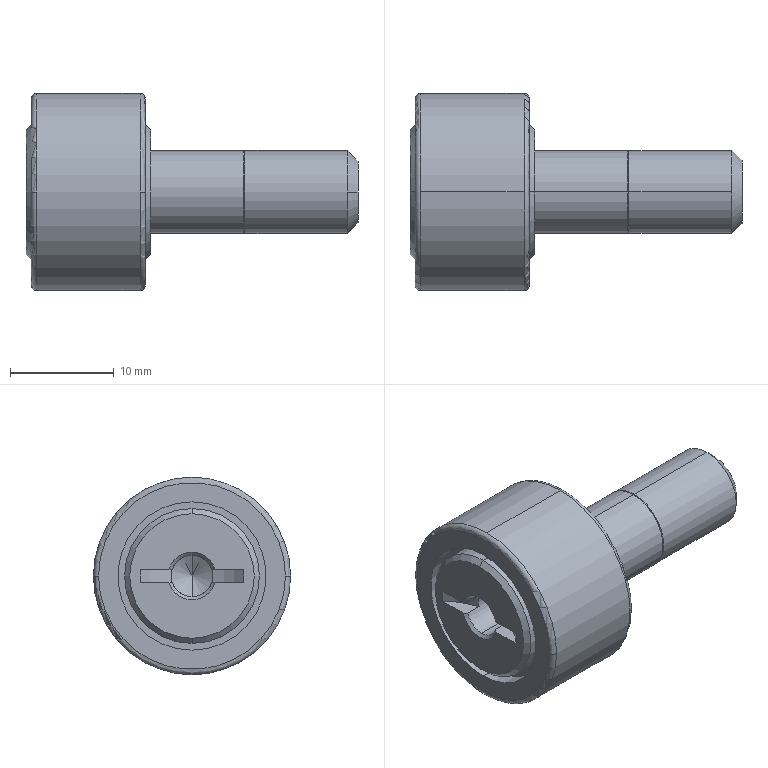Part | NX | 1 solid | 47 faces | box 32 x 19 x 19 mm | volume 4032 mm3 | cylinder 18 | cone 13 | plane 12 | torus 4 | commonest cylinder face diameters 8 x4 13 x4 14.3 x4 4 x2 14 x2 19 x2
STEP:
#1=CARTESIAN_POINT('',(32.,3.,0.));
#2=VERTEX_POINT('',#1);
#3=CARTESIAN_POINT('',(32.,-3.,0.));
#4=VERTEX_POINT('',#3);
#5=CARTESIAN_POINT('',(32.,0.,0.));
#6=DIRECTION('',(1.,0.,0.));
#7=DIRECTION('',(0.,0.,-1.));
#8=AXIS2_PLACEMENT_3D('',#5,#6,#7);
#9=CIRCLE('',#8,3.);
#10=EDGE_CURVE('',#2,#4,#9,.T.);
#11=ORIENTED_EDGE('',*,*,#10,.T.);
#12=CARTESIAN_POINT('',(32.,0.,0.));
#13=DIRECTION('',(1.,0.,0.));
#14=DIRECTION('',(0.,0.,-1.));
#15=AXIS2_PLACEMENT_3D('',#12,#13,#14);
#16=CIRCLE('',#15,3.);
#17=EDGE_CURVE('',#4,#2,#16,.T.);
#18=ORIENTED_EDGE('',*,*,#17,.T.);
#19=EDGE_LOOP('',(#11,#18));
#20=FACE_BOUND('',#19,.T.);
#21=CARTESIAN_POINT('',(32.,0.,0.));
#22=DIRECTION('',(1.,0.,0.));
#23=DIRECTION('',(0.,1.,0.));
#24=AXIS2_PLACEMENT_3D('',#21,#22,#23);
#25=PLANE('',#24);
#26=ADVANCED_FACE('',(#20),#25,.T.);
#27=CARTESIAN_POINT('',(31.,-4.,0.));
#28=VERTEX_POINT('',#27);
#29=CARTESIAN_POINT('',(31.,0.,4.));
#30=VERTEX_POINT('',#29);
#31=CARTESIAN_POINT('',(31.,0.,0.));
#32=DIRECTION('',(-1.,0.,0.));
#33=DIRECTION('',(0.,0.,-1.));
#34=AXIS2_PLACEMENT_3D('',#31,#32,#33);
#35=CIRCLE('',#34,4.);
#36=EDGE_CURVE('',#28,#30,#35,.T.);
#37=ORIENTED_EDGE('',*,*,#36,.F.);
#38=CARTESIAN_POINT('',(31.5,-3.5,0.));
#39=DIRECTION('',(-0.7071,-0.7071,0.));
#40=VECTOR('',#39,1000.);
#41=LINE('',#38,#40);
#42=EDGE_CURVE('',#4,#28,#41,.T.);
#43=ORIENTED_EDGE('',*,*,#42,.F.);
#44=ORIENTED_EDGE('',*,*,#10,.F.);
#45=CARTESIAN_POINT('',(31.,4.,0.));
#46=VERTEX_POINT('',#45);
#47=CARTESIAN_POINT('',(31.5,3.5,0.));
#48=DIRECTION('',(-0.7071,0.7071,0.));
#49=VECTOR('',#48,1000.);
#50=LINE('',#47,#49);
#51=EDGE_CURVE('',#2,#46,#50,.T.);
#52=ORIENTED_EDGE('',*,*,#51,.T.);
#53=CARTESIAN_POINT('',(31.,0.,0.));
#54=DIRECTION('',(-1.,0.,0.));
#55=DIRECTION('',(0.,0.,-1.));
#56=AXIS2_PLACEMENT_3D('',#53,#54,#55);
#57=CIRCLE('',#56,4.);
#58=EDGE_CURVE('',#30,#46,#57,.T.);
#59=ORIENTED_EDGE('',*,*,#58,.F.);
#60=EDGE_LOOP('',(#37,#43,#44,#52,#59));
#61=FACE_BOUND('',#60,.T.);
#62=CARTESIAN_POINT('',(31.5,0.,0.));
#63=DIRECTION('',(-1.,0.,0.));
#64=DIRECTION('',(0.,1.,0.));
#65=AXIS2_PLACEMENT_3D('',#62,#63,#64);
#66=CONICAL_SURFACE('',#65,3.5,0.7854);
#67=ADVANCED_FACE('',(#61),#66,.T.);
#68=CARTESIAN_POINT('',(0.5,0.,6.5));
#69=VERTEX_POINT('',#68);
#70=CARTESIAN_POINT('',(0.5,0.,-6.5));
#71=VERTEX_POINT('',#70);
#72=CARTESIAN_POINT('',(0.5,0.,0.));
#73=DIRECTION('',(-1.,0.,0.));
#74=DIRECTION('',(0.,0.,-1.));
#75=AXIS2_PLACEMENT_3D('',#72,#73,#74);
#76=CIRCLE('',#75,6.5);
#77=EDGE_CURVE('',#69,#71,#76,.T.);
#78=ORIENTED_EDGE('',*,*,#77,.F.);
#79=CARTESIAN_POINT('',(2.,0.,6.5));
#80=VERTEX_POINT('',#79);
#81=CARTESIAN_POINT('',(6.,0.,6.5));
#82=DIRECTION('',(-1.,0.,0.));
#83=VECTOR('',#82,1000.);
#84=LINE('',#81,#83);
#85=EDGE_CURVE('',#69,#80,#84,.F.);
#86=ORIENTED_EDGE('',*,*,#85,.T.);
#87=CARTESIAN_POINT('',(2.,0.,-6.5));
#88=VERTEX_POINT('',#87);
#89=CARTESIAN_POINT('',(2.,0.,0.));
#90=DIRECTION('',(1.,0.,0.));
#91=DIRECTION('',(0.,0.,-1.));
#92=AXIS2_PLACEMENT_3D('',#89,#90,#91);
#93=CIRCLE('',#92,6.5);
#94=EDGE_CURVE('',#88,#80,#93,.T.);
#95=ORIENTED_EDGE('',*,*,#94,.F.);
#96=CARTESIAN_POINT('',(6.,0.,-6.5));
#97=DIRECTION('',(-1.,0.,0.));
#98=VECTOR('',#97,1000.);
#99=LINE('',#96,#98);
#100=EDGE_CURVE('',#71,#88,#99,.F.);
#101=ORIENTED_EDGE('',*,*,#100,.F.);
#102=EDGE_LOOP('',(#78,#86,#95,#101));
#103=FACE_BOUND('',#102,.T.);
#104=CARTESIAN_POINT('',(6.,0.,0.));
#105=DIRECTION('',(-1.,0.,0.));
#106=DIRECTION('',(0.,0.,-1.));
#107=AXIS2_PLACEMENT_3D('',#104,#105,#106);
#108=CYLINDRICAL_SURFACE('',#107,6.5);
#109=ADVANCED_FACE('',(#103),#108,.T.);
#110=CARTESIAN_POINT('',(21.1,4.,0.));
#111=VERTEX_POINT('',#110);
#112=CARTESIAN_POINT('',(21.1,0.,4.));
#113=VERTEX_POINT('',#112);
#114=CARTESIAN_POINT('',(21.1,0.,0.));
#115=DIRECTION('',(1.,0.,0.));
#116=DIRECTION('',(0.,0.,-1.));
#117=AXIS2_PLACEMENT_3D('',#114,#115,#116);
#118=CIRCLE('',#117,4.);
#119=EDGE_CURVE('',#111,#113,#118,.T.);
#120=ORIENTED_EDGE('',*,*,#119,.T.);
#121=CARTESIAN_POINT('',(26.5,0.,4.));
#122=DIRECTION('',(1.,0.,0.));
#123=VECTOR('',#122,1000.);
#124=LINE('',#121,#123);
#125=EDGE_CURVE('',#113,#30,#124,.T.);
#126=ORIENTED_EDGE('',*,*,#125,.T.);
#127=ORIENTED_EDGE('',*,*,#58,.T.);
#128=CARTESIAN_POINT('',(31.,0.,-4.));
#129=VERTEX_POINT('',#128);
#130=CARTESIAN_POINT('',(31.,0.,0.));
#131=DIRECTION('',(-1.,0.,0.));
#132=DIRECTION('',(0.,0.,-1.));
#133=AXIS2_PLACEMENT_3D('',#130,#131,#132);
#134=CIRCLE('',#133,4.);
#135=EDGE_CURVE('',#46,#129,#134,.T.);
#136=ORIENTED_EDGE('',*,*,#135,.T.);
#137=CARTESIAN_POINT('',(21.1,0.,-4.));
#138=VERTEX_POINT('',#137);
#139=CARTESIAN_POINT('',(26.5,0.,-4.));
#140=DIRECTION('',(1.,0.,0.));
#141=VECTOR('',#140,1000.);
#142=LINE('',#139,#141);
#143=EDGE_CURVE('',#138,#129,#142,.T.);
#144=ORIENTED_EDGE('',*,*,#143,.F.);
#145=CARTESIAN_POINT('',(21.1,0.,0.));
#146=DIRECTION('',(1.,0.,0.));
#147=DIRECTION('',(0.,0.,-1.));
#148=AXIS2_PLACEMENT_3D('',#145,#146,#147);
#149=CIRCLE('',#148,4.);
#150=EDGE_CURVE('',#138,#111,#149,.T.);
#151=ORIENTED_EDGE('',*,*,#150,.T.);
#152=EDGE_LOOP('',(#120,#126,#127,#136,#144,#151));
#153=FACE_BOUND('',#152,.T.);
#154=CARTESIAN_POINT('',(26.5,0.,0.));
#155=DIRECTION('',(1.,0.,0.));
#156=DIRECTION('',(0.,0.,-1.));
#157=AXIS2_PLACEMENT_3D('',#154,#155,#156);
#158=CYLINDRICAL_SURFACE('',#157,4.);
#159=ADVANCED_FACE('',(#153),#158,.T.);
#160=CARTESIAN_POINT('',(2.,0.,-7.15));
#161=VERTEX_POINT('',#160);
#162=CARTESIAN_POINT('',(2.,0.,7.15));
#163=VERTEX_POINT('',#162);
#164=CARTESIAN_POINT('',(2.,0.,0.));
#165=DIRECTION('',(1.,0.,0.));
#166=DIRECTION('',(0.,0.,-1.));
#167=AXIS2_PLACEMENT_3D('',#164,#165,#166);
#168=CIRCLE('',#167,7.15);
#169=EDGE_CURVE('',#161,#163,#168,.T.);
#170=ORIENTED_EDGE('',*,*,#169,.F.);
#171=CARTESIAN_POINT('',(2.,0.,0.));
#172=DIRECTION('',(1.,0.,0.));
#173=DIRECTION('',(0.,0.,-1.));
#174=AXIS2_PLACEMENT_3D('',#171,#172,#173);
#175=CIRCLE('',#174,7.15);
#176=EDGE_CURVE('',#163,#161,#175,.T.);
#177=ORIENTED_EDGE('',*,*,#176,.F.);
#178=EDGE_LOOP('',(#170,#177));
#179=FACE_BOUND('',#178,.T.);
#180=ORIENTED_EDGE('',*,*,#94,.T.);
#181=CARTESIAN_POINT('',(2.,0.,0.));
#182=DIRECTION('',(1.,0.,0.));
#183=DIRECTION('',(0.,0.,-1.));
#184=AXIS2_PLACEMENT_3D('',#181,#182,#183);
#185=CIRCLE('',#184,6.5);
#186=EDGE_CURVE('',#80,#88,#185,.T.);
#187=ORIENTED_EDGE('',*,*,#186,.T.);
#188=EDGE_LOOP('',(#180,#187));
#189=FACE_BOUND('',#188,.T.);
#190=CARTESIAN_POINT('',(2.,0.,0.));
#191=DIRECTION('',(1.,0.,0.));
#192=DIRECTION('',(0.,0.,1.));
#193=AXIS2_PLACEMENT_3D('',#190,#191,#192);
#194=PLANE('',#193);
#195=ADVANCED_FACE('',(#179,#189),#194,.F.);
#196=ORIENTED_EDGE('',*,*,#119,.F.);
#197=CARTESIAN_POINT('',(21.,3.9,0.));
#198=VERTEX_POINT('',#197);
#199=CARTESIAN_POINT('',(21.05,3.95,0.));
#200=DIRECTION('',(0.7071,0.7071,0.));
#201=VECTOR('',#200,1000.);
#202=LINE('',#199,#201);
#203=EDGE_CURVE('',#198,#111,#202,.T.);
#204=ORIENTED_EDGE('',*,*,#203,.F.);
#205=CARTESIAN_POINT('',(21.,-3.9,0.));
#206=VERTEX_POINT('',#205);
#207=CARTESIAN_POINT('',(21.,0.,0.));
#208=DIRECTION('',(-1.,0.,0.));
#209=DIRECTION('',(0.,0.,-1.));
#210=AXIS2_PLACEMENT_3D('',#207,#208,#209);
#211=CIRCLE('',#210,3.9);
#212=EDGE_CURVE('',#206,#198,#211,.T.);
#213=ORIENTED_EDGE('',*,*,#212,.F.);
#214=CARTESIAN_POINT('',(21.1,-4.,0.));
#215=VERTEX_POINT('',#214);
#216=CARTESIAN_POINT('',(21.05,-3.95,0.));
#217=DIRECTION('',(0.7071,-0.7071,0.));
#218=VECTOR('',#217,1000.);
#219=LINE('',#216,#218);
#220=EDGE_CURVE('',#206,#215,#219,.T.);
#221=ORIENTED_EDGE('',*,*,#220,.T.);
#222=CARTESIAN_POINT('',(21.1,0.,0.));
#223=DIRECTION('',(1.,0.,0.));
#224=DIRECTION('',(0.,0.,-1.));
#225=AXIS2_PLACEMENT_3D('',#222,#223,#224);
#226=CIRCLE('',#225,4.);
#227=EDGE_CURVE('',#113,#215,#226,.T.);
#228=ORIENTED_EDGE('',*,*,#227,.F.);
#229=EDGE_LOOP('',(#196,#204,#213,#221,#228));
#230=FACE_BOUND('',#229,.T.);
#231=CARTESIAN_POINT('',(21.05,0.,0.));
#232=DIRECTION('',(1.,0.,0.));
#233=DIRECTION('',(0.,-1.,0.));
#234=AXIS2_PLACEMENT_3D('',#231,#232,#233);
#235=CONICAL_SURFACE('',#234,3.95,0.7854);
#236=ADVANCED_FACE('',(#230),#235,.T.);
#237=CARTESIAN_POINT('',(11.5,-9.,0.));
#238=VERTEX_POINT('',#237);
#239=CARTESIAN_POINT('',(11.5,9.,0.));
#240=VERTEX_POINT('',#239);
#241=CARTESIAN_POINT('',(11.5,0.,0.));
#242=DIRECTION('',(-1.,0.,0.));
#243=DIRECTION('',(0.,0.,-1.));
#244=AXIS2_PLACEMENT_3D('',#241,#242,#243);
#245=CIRCLE('',#244,9.);
#246=EDGE_CURVE('',#238,#240,#245,.T.);
#247=ORIENTED_EDGE('',*,*,#246,.F.);
#248=CARTESIAN_POINT('',(11.5,0.,0.));
#249=DIRECTION('',(-1.,0.,0.));
#250=DIRECTION('',(0.,0.,-1.));
#251=AXIS2_PLACEMENT_3D('',#248,#249,#250);
#252=CIRCLE('',#251,9.);
#253=EDGE_CURVE('',#240,#238,#252,.T.);
#254=ORIENTED_EDGE('',*,*,#253,.F.);
#255=EDGE_LOOP('',(#247,#254));
#256=FACE_BOUND('',#255,.T.);
#257=CARTESIAN_POINT('',(11.5,0.,-7.15));
#258=VERTEX_POINT('',#257);
#259=CARTESIAN_POINT('',(11.5,0.,7.15));
#260=VERTEX_POINT('',#259);
#261=CARTESIAN_POINT('',(11.5,0.,0.));
#262=DIRECTION('',(-1.,0.,0.));
#263=DIRECTION('',(0.,0.,1.));
#264=AXIS2_PLACEMENT_3D('',#261,#262,#263);
#265=CIRCLE('',#264,7.15);
#266=EDGE_CURVE('',#258,#260,#265,.T.);
#267=ORIENTED_EDGE('',*,*,#266,.T.);
#268=CARTESIAN_POINT('',(11.5,0.,0.));
#269=DIRECTION('',(-1.,0.,0.));
#270=DIRECTION('',(0.,0.,1.));
#271=AXIS2_PLACEMENT_3D('',#268,#269,#270);
#272=CIRCLE('',#271,7.15);
#273=EDGE_CURVE('',#260,#258,#272,.T.);
#274=ORIENTED_EDGE('',*,*,#273,.T.);
#275=EDGE_LOOP('',(#267,#274));
#276=FACE_BOUND('',#275,.T.);
#277=CARTESIAN_POINT('',(11.5,0.,-4.5));
#278=DIRECTION('',(1.,0.,0.));
#279=DIRECTION('',(0.,1.,0.));
#280=AXIS2_PLACEMENT_3D('',#277,#278,#279);
#281=PLANE('',#280);
#282=ADVANCED_FACE('',(#256,#276),#281,.T.);
#283=CARTESIAN_POINT('',(8.,0.,-2.));
#284=VERTEX_POINT('',#283);
#285=CARTESIAN_POINT('',(8.,0.,2.));
#286=VERTEX_POINT('',#285);
#287=CARTESIAN_POINT('',(8.,0.,0.));
#288=DIRECTION('',(-1.,0.,0.));
#289=DIRECTION('',(0.,0.,-1.));
#290=AXIS2_PLACEMENT_3D('',#287,#288,#289);
#291=CIRCLE('',#290,2.);
#292=EDGE_CURVE('',#284,#286,#291,.T.);
#293=ORIENTED_EDGE('',*,*,#292,.T.);
#294=CARTESIAN_POINT('',(9.155,0.,0.));
#295=VERTEX_POINT('',#294);
#296=CARTESIAN_POINT('',(8.577,0.,1.));
#297=DIRECTION('',(-0.5,0.,0.866));
#298=VECTOR('',#297,1000.);
#299=LINE('',#296,#298);
#300=EDGE_CURVE('',#286,#295,#299,.F.);
#301=ORIENTED_EDGE('',*,*,#300,.T.);
#302=CARTESIAN_POINT('',(8.577,0.,-1.));
#303=DIRECTION('',(-0.5,0.,-0.866));
#304=VECTOR('',#303,1000.);
#305=LINE('',#302,#304);
#306=EDGE_CURVE('',#284,#295,#305,.F.);
#307=ORIENTED_EDGE('',*,*,#306,.F.);
#308=EDGE_LOOP('',(#293,#301,#307));
#309=FACE_BOUND('',#308,.T.);
#310=CARTESIAN_POINT('',(8.577,0.,0.));
#311=DIRECTION('',(-1.,0.,0.));
#312=DIRECTION('',(0.,0.,1.));
#313=AXIS2_PLACEMENT_3D('',#310,#311,#312);
#314=CONICAL_SURFACE('',#313,1.,1.047);
#315=ADVANCED_FACE('',(#309),#314,.F.);
#316=CARTESIAN_POINT('',(10.,0.,-7.15));
#317=VERTEX_POINT('',#316);
#318=CARTESIAN_POINT('',(10.,0.,7.15));
#319=VERTEX_POINT('',#318);
#320=CARTESIAN_POINT('',(10.,0.,0.));
#321=DIRECTION('',(-1.,0.,0.));
#322=DIRECTION('',(0.,0.,1.));
#323=AXIS2_PLACEMENT_3D('',#320,#321,#322);
#324=CIRCLE('',#323,7.15);
#325=EDGE_CURVE('',#317,#319,#324,.T.);
#326=ORIENTED_EDGE('',*,*,#325,.T.);
#327=CARTESIAN_POINT('',(11.,0.,7.15));
#328=DIRECTION('',(-1.,0.,0.));
#329=VECTOR('',#328,1000.);
#330=LINE('',#327,#329);
#331=EDGE_CURVE('',#260,#319,#330,.T.);
#332=ORIENTED_EDGE('',*,*,#331,.F.);
#333=ORIENTED_EDGE('',*,*,#266,.F.);
#334=CARTESIAN_POINT('',(11.,0.,-7.15));
#335=DIRECTION('',(-1.,0.,0.));
#336=VECTOR('',#335,1000.);
#337=LINE('',#334,#336);
#338=EDGE_CURVE('',#258,#317,#337,.T.);
#339=ORIENTED_EDGE('',*,*,#338,.T.);
#340=EDGE_LOOP('',(#326,#332,#333,#339));
#341=FACE_BOUND('',#340,.T.);
#342=CARTESIAN_POINT('',(11.,0.,0.));
#343=DIRECTION('',(-1.,0.,0.));
#344=DIRECTION('',(0.,0.,1.));
#345=AXIS2_PLACEMENT_3D('',#342,#343,#344);
#346=CYLINDRICAL_SURFACE('',#345,7.15);
#347=ADVANCED_FACE('',(#341),#346,.F.);
#348=CARTESIAN_POINT('',(21.,0.,4.));
#349=VERTEX_POINT('',#348);
#350=CARTESIAN_POINT('',(21.,0.,-4.));
#351=VERTEX_POINT('',#350);
#352=CARTESIAN_POINT('',(21.,0.,0.));
#353=DIRECTION('',(1.,0.,0.));
#354=DIRECTION('',(0.,0.,-1.));
#355=AXIS2_PLACEMENT_3D('',#352,#353,#354);
#356=CIRCLE('',#355,4.);
#357=EDGE_CURVE('',#349,#351,#356,.T.);
#358=ORIENTED_EDGE('',*,*,#357,.T.);
#359=CARTESIAN_POINT('',(21.,0.,0.));
#360=DIRECTION('',(1.,0.,0.));
#361=DIRECTION('',(0.,0.,-1.));
#362=AXIS2_PLACEMENT_3D('',#359,#360,#361);
#363=CIRCLE('',#362,4.);
#364=EDGE_CURVE('',#351,#349,#363,.T.);
#365=ORIENTED_EDGE('',*,*,#364,.T.);
#366=EDGE_LOOP('',(#358,#365));
#367=FACE_BOUND('',#366,.T.);
#368=CARTESIAN_POINT('',(21.,0.,0.));
#369=DIRECTION('',(-1.,0.,0.));
#370=DIRECTION('',(0.,0.,-1.));
#371=AXIS2_PLACEMENT_3D('',#368,#369,#370);
#372=CIRCLE('',#371,3.9);
#373=EDGE_CURVE('',#198,#206,#372,.T.);
#374=ORIENTED_EDGE('',*,*,#373,.T.);
#375=ORIENTED_EDGE('',*,*,#212,.T.);
#376=EDGE_LOOP('',(#374,#375));
#377=FACE_BOUND('',#376,.T.);
#378=CARTESIAN_POINT('',(21.,0.,0.));
#379=DIRECTION('',(1.,0.,0.));
#380=DIRECTION('',(0.,1.,0.));
#381=AXIS2_PLACEMENT_3D('',#378,#379,#380);
#382=PLANE('',#381);
#383=ADVANCED_FACE('',(#367,#377),#382,.T.);
#384=ORIENTED_EDGE('',*,*,#292,.F.);
#385=CARTESIAN_POINT('',(0.3,0.,-2.));
#386=VERTEX_POINT('',#385);
#387=CARTESIAN_POINT('',(4.15,0.,-2.));
#388=DIRECTION('',(-1.,0.,0.));
#389=VECTOR('',#388,1000.);
#390=LINE('',#387,#389);
#391=EDGE_CURVE('',#386,#284,#390,.F.);
#392=ORIENTED_EDGE('',*,*,#391,.F.);
#393=CARTESIAN_POINT('',(0.3,-1.908,-0.6));
#394=VERTEX_POINT('',#393);
#395=CARTESIAN_POINT('',(0.3,0.,0.));
#396=DIRECTION('',(-1.,0.,0.));
#397=DIRECTION('',(0.,0.,-1.));
#398=AXIS2_PLACEMENT_3D('',#395,#396,#397);
#399=CIRCLE('',#398,2.);
#400=EDGE_CURVE('',#386,#394,#399,.T.);
#401=ORIENTED_EDGE('',*,*,#400,.T.);
#402=CARTESIAN_POINT('',(1.836,-1.908,-0.6));
#403=VERTEX_POINT('',#402);
#404=CARTESIAN_POINT('',(4.15,-1.908,-0.6));
#405=DIRECTION('',(1.,0.,0.));
#406=VECTOR('',#405,1000.);
#407=LINE('',#404,#406);
#408=EDGE_CURVE('',#394,#403,#407,.T.);
#409=ORIENTED_EDGE('',*,*,#408,.T.);
#410=CARTESIAN_POINT('',(1.836,-1.908,0.6));
#411=VERTEX_POINT('',#410);
#412=CARTESIAN_POINT('',(1.836,-1.908,-0.6));
#413=CARTESIAN_POINT('',(1.832,-1.923,-0.5515));
#414=CARTESIAN_POINT('',(1.828,-1.936,-0.5025));
#415=CARTESIAN_POINT('',(1.825,-1.948,-0.4532));
#416=CARTESIAN_POINT('',(1.823,-1.954,-0.4286));
#417=CARTESIAN_POINT('',(1.821,-1.959,-0.4038));
#418=CARTESIAN_POINT('',(1.82,-1.964,-0.379));
#419=CARTESIAN_POINT('',(1.819,-1.969,-0.3542));
#420=CARTESIAN_POINT('',(1.817,-1.973,-0.3293));
#421=CARTESIAN_POINT('',(1.816,-1.977,-0.3043));
#422=CARTESIAN_POINT('',(1.814,-1.984,-0.2543));
#423=CARTESIAN_POINT('',(1.812,-1.99,-0.2037));
#424=CARTESIAN_POINT('',(1.811,-1.994,-0.1529));
#425=CARTESIAN_POINT('',(1.81,-1.996,-0.1275));
#426=CARTESIAN_POINT('',(1.81,-1.998,-0.1021));
#427=CARTESIAN_POINT('',(1.81,-1.999,-0.07658));
#428=CARTESIAN_POINT('',(1.809,-2.,-0.05109));
#429=CARTESIAN_POINT('',(1.809,-2.,-0.02556));
#430=CARTESIAN_POINT('',(1.809,-2.,-0.00003605));
#431=CARTESIAN_POINT('',(1.809,-2.,0.02549));
#432=CARTESIAN_POINT('',(1.809,-2.,0.05102));
#433=CARTESIAN_POINT('',(1.81,-1.999,0.07653));
#434=CARTESIAN_POINT('',(1.81,-1.998,0.102));
#435=CARTESIAN_POINT('',(1.81,-1.996,0.1275));
#436=CARTESIAN_POINT('',(1.811,-1.994,0.1529));
#437=CARTESIAN_POINT('',(1.812,-1.99,0.2038));
#438=CARTESIAN_POINT('',(1.814,-1.984,0.2543));
#439=CARTESIAN_POINT('',(1.816,-1.977,0.3045));
#440=CARTESIAN_POINT('',(1.817,-1.973,0.3295));
#441=CARTESIAN_POINT('',(1.819,-1.968,0.3545));
#442=CARTESIAN_POINT('',(1.82,-1.964,0.3793));
#443=CARTESIAN_POINT('',(1.821,-1.959,0.4041));
#444=CARTESIAN_POINT('',(1.823,-1.954,0.4287));
#445=CARTESIAN_POINT('',(1.825,-1.948,0.4534));
#446=CARTESIAN_POINT('',(1.828,-1.936,0.5026));
#447=CARTESIAN_POINT('',(1.832,-1.923,0.5516));
#448=CARTESIAN_POINT('',(1.836,-1.908,0.6));
#449=B_SPLINE_CURVE_WITH_KNOTS('',3,(#412,#413,#414,#415,#416,#417,#418,#419,#420,#421,#422,#423,#424,#425,#426,#427,#428,#429,#430,#431,#432,#433,#434,#435,#436,#437,#438,#439,#440,#441,#442,#443,#444,#445,#446,#447,#448),.UNSPECIFIED.,.F.,.F.,(4,3,3,3,3,3,3,3,3,3,3,3,4),(0.,0.1526,0.2287,0.3046,0.4571,0.5336,0.6101,0.6867,0.7632,0.9159,0.9919,1.068,1.22),.UNSPECIFIED.);
#450=EDGE_CURVE('',#403,#411,#449,.T.);
#451=ORIENTED_EDGE('',*,*,#450,.T.);
#452=CARTESIAN_POINT('',(0.3,-1.908,0.6));
#453=VERTEX_POINT('',#452);
#454=CARTESIAN_POINT('',(4.15,-1.908,0.6));
#455=DIRECTION('',(-1.,0.,0.));
#456=VECTOR('',#455,1000.);
#457=LINE('',#454,#456);
#458=EDGE_CURVE('',#411,#453,#457,.T.);
#459=ORIENTED_EDGE('',*,*,#458,.T.);
#460=CARTESIAN_POINT('',(0.3,0.,2.));
#461=VERTEX_POINT('',#460);
#462=CARTESIAN_POINT('',(0.3,0.,0.));
#463=DIRECTION('',(-1.,0.,0.));
#464=DIRECTION('',(0.,0.,-1.));
#465=AXIS2_PLACEMENT_3D('',#462,#463,#464);
#466=CIRCLE('',#465,2.);
#467=EDGE_CURVE('',#453,#461,#466,.T.);
#468=ORIENTED_EDGE('',*,*,#467,.T.);
#469=CARTESIAN_POINT('',(4.15,0.,2.));
#470=DIRECTION('',(-1.,0.,0.));
#471=VECTOR('',#470,1000.);
#472=LINE('',#469,#471);
#473=EDGE_CURVE('',#461,#286,#472,.F.);
#474=ORIENTED_EDGE('',*,*,#473,.T.);
#475=EDGE_LOOP('',(#384,#392,#401,#409,#451,#459,#468,#474));
#476=FACE_BOUND('',#475,.T.);
#477=CARTESIAN_POINT('',(4.15,0.,0.));
#478=DIRECTION('',(-1.,0.,0.));
#479=DIRECTION('',(0.,0.,-1.));
#480=AXIS2_PLACEMENT_3D('',#477,#478,#479);
#481=CYLINDRICAL_SURFACE('',#480,2.);
#482=ADVANCED_FACE('',(#476),#481,.F.);
#483=ORIENTED_EDGE('',*,*,#325,.F.);
#484=CARTESIAN_POINT('',(10.,0.,0.));
#485=DIRECTION('',(-1.,0.,0.));
#486=DIRECTION('',(0.,0.,1.));
#487=AXIS2_PLACEMENT_3D('',#484,#485,#486);
#488=CIRCLE('',#487,7.15);
#489=EDGE_CURVE('',#319,#317,#488,.T.);
#490=ORIENTED_EDGE('',*,*,#489,.F.);
#491=EDGE_LOOP('',(#483,#490));
#492=FACE_BOUND('',#491,.T.);
#493=CARTESIAN_POINT('',(10.,0.,-6.5));
#494=VERTEX_POINT('',#493);
#495=CARTESIAN_POINT('',(10.,0.,6.5));
#496=VERTEX_POINT('',#495);
#497=CARTESIAN_POINT('',(10.,0.,0.));
#498=DIRECTION('',(-1.,0.,0.));
#499=DIRECTION('',(0.,0.,-1.));
#500=AXIS2_PLACEMENT_3D('',#497,#498,#499);
#501=CIRCLE('',#500,6.5);
#502=EDGE_CURVE('',#494,#496,#501,.T.);
#503=ORIENTED_EDGE('',*,*,#502,.T.);
#504=CARTESIAN_POINT('',(10.,0.,0.));
#505=DIRECTION('',(-1.,0.,0.));
#506=DIRECTION('',(0.,0.,-1.));
#507=AXIS2_PLACEMENT_3D('',#504,#505,#506);
#508=CIRCLE('',#507,6.5);
#509=EDGE_CURVE('',#496,#494,#508,.T.);
#510=ORIENTED_EDGE('',*,*,#509,.T.);
#511=EDGE_LOOP('',(#503,#510));
#512=FACE_BOUND('',#511,.T.);
#513=CARTESIAN_POINT('',(10.,0.,0.));
#514=DIRECTION('',(-1.,0.,0.));
#515=DIRECTION('',(0.,0.,1.));
#516=AXIS2_PLACEMENT_3D('',#513,#514,#515);
#517=PLANE('',#516);
#518=ADVANCED_FACE('',(#492,#512),#517,.F.);
#519=ORIENTED_EDGE('',*,*,#357,.F.);
#520=CARTESIAN_POINT('',(12.,0.,4.));
#521=VERTEX_POINT('',#520);
#522=CARTESIAN_POINT('',(16.5,0.,4.));
#523=DIRECTION('',(1.,0.,0.));
#524=VECTOR('',#523,1000.);
#525=LINE('',#522,#524);
#526=EDGE_CURVE('',#521,#349,#525,.T.);
#527=ORIENTED_EDGE('',*,*,#526,.F.);
#528=CARTESIAN_POINT('',(12.,0.,-4.));
#529=VERTEX_POINT('',#528);
#530=CARTESIAN_POINT('',(12.,0.,0.));
#531=DIRECTION('',(-1.,0.,0.));
#532=DIRECTION('',(0.,0.,-1.));
#533=AXIS2_PLACEMENT_3D('',#530,#531,#532);
#534=CIRCLE('',#533,4.);
#535=EDGE_CURVE('',#529,#521,#534,.T.);
#536=ORIENTED_EDGE('',*,*,#535,.F.);
#537=CARTESIAN_POINT('',(16.5,0.,-4.));
#538=DIRECTION('',(1.,0.,0.));
#539=VECTOR('',#538,1000.);
#540=LINE('',#537,#539);
#541=EDGE_CURVE('',#529,#351,#540,.T.);
#542=ORIENTED_EDGE('',*,*,#541,.T.);
#543=EDGE_LOOP('',(#519,#527,#536,#542));
#544=FACE_BOUND('',#543,.T.);
#545=CARTESIAN_POINT('',(16.5,0.,0.));
#546=DIRECTION('',(1.,0.,0.));
#547=DIRECTION('',(0.,0.,-1.));
#548=AXIS2_PLACEMENT_3D('',#545,#546,#547);
#549=CYLINDRICAL_SURFACE('',#548,4.);
#550=ADVANCED_FACE('',(#544),#549,.T.);
#551=CARTESIAN_POINT('',(0.5,-9.,0.));
#552=VERTEX_POINT('',#551);
#553=CARTESIAN_POINT('',(0.5,9.,0.));
#554=VERTEX_POINT('',#553);
#555=CARTESIAN_POINT('',(0.5,0.,0.));
#556=DIRECTION('',(1.,0.,0.));
#557=DIRECTION('',(0.,0.,1.));
#558=AXIS2_PLACEMENT_3D('',#555,#556,#557);
#559=CIRCLE('',#558,9.);
#560=EDGE_CURVE('',#552,#554,#559,.T.);
#561=ORIENTED_EDGE('',*,*,#560,.T.);
#562=CARTESIAN_POINT('',(1.,9.5,0.));
#563=VERTEX_POINT('',#562);
#564=CARTESIAN_POINT('',(1.,9.,0.));
#565=DIRECTION('',(0.,0.,1.));
#566=DIRECTION('',(-1.,0.,0.));
#567=AXIS2_PLACEMENT_3D('',#564,#565,#566);
#568=CIRCLE('',#567,0.5);
#569=EDGE_CURVE('',#554,#563,#568,.F.);
#570=ORIENTED_EDGE('',*,*,#569,.T.);
#571=CARTESIAN_POINT('',(1.,0.,-9.5));
#572=VERTEX_POINT('',#571);
#573=CARTESIAN_POINT('',(1.,0.,0.));
#574=DIRECTION('',(1.,0.,0.));
#575=DIRECTION('',(0.,0.,1.));
#576=AXIS2_PLACEMENT_3D('',#573,#574,#575);
#577=CIRCLE('',#576,9.5);
#578=EDGE_CURVE('',#572,#563,#577,.T.);
#579=ORIENTED_EDGE('',*,*,#578,.F.);
#580=CARTESIAN_POINT('',(1.,-9.5,0.));
#581=VERTEX_POINT('',#580);
#582=CARTESIAN_POINT('',(1.,0.,0.));
#583=DIRECTION('',(1.,0.,0.));
#584=DIRECTION('',(0.,0.,1.));
#585=AXIS2_PLACEMENT_3D('',#582,#583,#584);
#586=CIRCLE('',#585,9.5);
#587=EDGE_CURVE('',#581,#572,#586,.T.);
#588=ORIENTED_EDGE('',*,*,#587,.F.);
#589=CARTESIAN_POINT('',(1.,-9.,0.));
#590=DIRECTION('',(0.,0.,-1.));
#591=DIRECTION('',(-1.,0.,0.));
#592=AXIS2_PLACEMENT_3D('',#589,#590,#591);
#593=CIRCLE('',#592,0.5);
#594=EDGE_CURVE('',#552,#581,#593,.F.);
#595=ORIENTED_EDGE('',*,*,#594,.F.);
#596=EDGE_LOOP('',(#561,#570,#579,#588,#595));
#597=FACE_BOUND('',#596,.T.);
#598=CARTESIAN_POINT('',(1.,0.,0.));
#599=DIRECTION('',(1.,0.,0.));
#600=DIRECTION('',(0.,-1.,0.));
#601=AXIS2_PLACEMENT_3D('',#598,#599,#600);
#602=TOROIDAL_SURFACE('',#601,9.,0.5);
#603=ADVANCED_FACE('',(#597),#602,.T.);
#604=CARTESIAN_POINT('',(1.836,1.908,0.6));
#605=VERTEX_POINT('',#604);
#606=CARTESIAN_POINT('',(1.836,1.908,-0.6));
#607=VERTEX_POINT('',#606);
#608=CARTESIAN_POINT('',(1.836,1.908,0.6));
#609=CARTESIAN_POINT('',(1.832,1.923,0.5515));
#610=CARTESIAN_POINT('',(1.828,1.936,0.5025));
#611=CARTESIAN_POINT('',(1.825,1.948,0.4532));
#612=CARTESIAN_POINT('',(1.823,1.954,0.4286));
#613=CARTESIAN_POINT('',(1.821,1.959,0.4038));
#614=CARTESIAN_POINT('',(1.82,1.964,0.379));
#615=CARTESIAN_POINT('',(1.819,1.969,0.3542));
#616=CARTESIAN_POINT('',(1.817,1.973,0.3293));
#617=CARTESIAN_POINT('',(1.816,1.977,0.3043));
#618=CARTESIAN_POINT('',(1.814,1.984,0.2543));
#619=CARTESIAN_POINT('',(1.812,1.99,0.2037));
#620=CARTESIAN_POINT('',(1.811,1.994,0.1529));
#621=CARTESIAN_POINT('',(1.81,1.996,0.1275));
#622=CARTESIAN_POINT('',(1.81,1.998,0.1021));
#623=CARTESIAN_POINT('',(1.81,1.999,0.07658));
#624=CARTESIAN_POINT('',(1.809,2.,0.05109));
#625=CARTESIAN_POINT('',(1.809,2.,0.02556));
#626=CARTESIAN_POINT('',(1.809,2.,0.00003605));
#627=CARTESIAN_POINT('',(1.809,2.,-0.02549));
#628=CARTESIAN_POINT('',(1.809,2.,-0.05102));
#629=CARTESIAN_POINT('',(1.81,1.999,-0.07653));
#630=CARTESIAN_POINT('',(1.81,1.998,-0.102));
#631=CARTESIAN_POINT('',(1.81,1.996,-0.1275));
#632=CARTESIAN_POINT('',(1.811,1.994,-0.1529));
#633=CARTESIAN_POINT('',(1.812,1.99,-0.2038));
#634=CARTESIAN_POINT('',(1.814,1.984,-0.2543));
#635=CARTESIAN_POINT('',(1.816,1.977,-0.3045));
#636=CARTESIAN_POINT('',(1.817,1.973,-0.3295));
#637=CARTESIAN_POINT('',(1.819,1.968,-0.3545));
#638=CARTESIAN_POINT('',(1.82,1.964,-0.3793));
#639=CARTESIAN_POINT('',(1.821,1.959,-0.4041));
#640=CARTESIAN_POINT('',(1.823,1.954,-0.4287));
#641=CARTESIAN_POINT('',(1.825,1.948,-0.4534));
#642=CARTESIAN_POINT('',(1.828,1.936,-0.5026));
#643=CARTESIAN_POINT('',(1.832,1.923,-0.5516));
#644=CARTESIAN_POINT('',(1.836,1.908,-0.6));
#645=B_SPLINE_CURVE_WITH_KNOTS('',3,(#608,#609,#610,#611,#612,#613,#614,#615,#616,#617,#618,#619,#620,#621,#622,#623,#624,#625,#626,#627,#628,#629,#630,#631,#632,#633,#634,#635,#636,#637,#638,#639,#640,#641,#642,#643,#644),.UNSPECIFIED.,.F.,.F.,(4,3,3,3,3,3,3,3,3,3,3,3,4),(0.,0.1526,0.2287,0.3046,0.4571,0.5336,0.6101,0.6867,0.7632,0.9159,0.9919,1.068,1.22),.UNSPECIFIED.);
#646=EDGE_CURVE('',#605,#607,#645,.T.);
#647=ORIENTED_EDGE('',*,*,#646,.F.);
#648=CARTESIAN_POINT('',(0.,5.,0.6));
#649=VERTEX_POINT('',#648);
#650=CARTESIAN_POINT('',(-4.899,0.,0.6));
#651=DIRECTION('',(0.,0.,1.));
#652=DIRECTION('',(1.,0.,0.));
#653=AXIS2_PLACEMENT_3D('',#650,#651,#652);
#654=CIRCLE('',#653,7.);
#655=EDGE_CURVE('',#605,#649,#654,.T.);
#656=ORIENTED_EDGE('',*,*,#655,.T.);
#657=CARTESIAN_POINT('',(0.,5.,-0.6));
#658=VERTEX_POINT('',#657);
#659=CARTESIAN_POINT('',(0.,5.,0.));
#660=DIRECTION('',(0.,0.,1.));
#661=VECTOR('',#660,1000.);
#662=LINE('',#659,#661);
#663=EDGE_CURVE('',#658,#649,#662,.T.);
#664=ORIENTED_EDGE('',*,*,#663,.F.);
#665=CARTESIAN_POINT('',(-4.899,0.,-0.6));
#666=DIRECTION('',(0.,0.,-1.));
#667=DIRECTION('',(1.,0.,0.));
#668=AXIS2_PLACEMENT_3D('',#665,#666,#667);
#669=CIRCLE('',#668,7.);
#670=EDGE_CURVE('',#658,#607,#669,.T.);
#671=ORIENTED_EDGE('',*,*,#670,.T.);
#672=EDGE_LOOP('',(#647,#656,#664,#671));
#673=FACE_BOUND('',#672,.T.);
#674=CARTESIAN_POINT('',(-4.899,0.,0.));
#675=DIRECTION('',(0.,0.,1.));
#676=DIRECTION('',(1.,0.,0.));
#677=AXIS2_PLACEMENT_3D('',#674,#675,#676);
#678=CYLINDRICAL_SURFACE('',#677,7.);
#679=ADVANCED_FACE('',(#673),#678,.F.);
#680=CARTESIAN_POINT('',(0.3,1.908,-0.6));
#681=VERTEX_POINT('',#680);
#682=CARTESIAN_POINT('',(4.15,1.908,-0.6));
#683=DIRECTION('',(-1.,0.,0.));
#684=VECTOR('',#683,1000.);
#685=LINE('',#682,#684);
#686=EDGE_CURVE('',#607,#681,#685,.T.);
#687=ORIENTED_EDGE('',*,*,#686,.F.);
#688=ORIENTED_EDGE('',*,*,#670,.F.);
#689=CARTESIAN_POINT('',(0.,2.22,-0.6));
#690=VERTEX_POINT('',#689);
#691=CARTESIAN_POINT('',(0.,0.,-0.6));
#692=DIRECTION('',(0.,1.,0.));
#693=VECTOR('',#692,1000.);
#694=LINE('',#691,#693);
#695=EDGE_CURVE('',#690,#658,#694,.T.);
#696=ORIENTED_EDGE('',*,*,#695,.F.);
#697=CARTESIAN_POINT('',(0.3,1.908,-0.6));
#698=CARTESIAN_POINT('',(0.1614,2.053,-0.6));
#699=CARTESIAN_POINT('',(0.,2.22,-0.6));
#700=(BOUNDED_CURVE()B_SPLINE_CURVE(2,(#697,#698,#699),.UNSPECIFIED.,.F.,.F.)B_SPLINE_CURVE_WITH_KNOTS((3,3),(0.,0.4332),.UNSPECIFIED.)CURVE()GEOMETRIC_REPRESENTATION_ITEM()RATIONAL_B_SPLINE_CURVE((1.,1.003,1.))REPRESENTATION_ITEM(''));
#701=EDGE_CURVE('',#681,#690,#700,.T.);
#702=ORIENTED_EDGE('',*,*,#701,.F.);
#703=EDGE_LOOP('',(#687,#688,#696,#702));
#704=FACE_BOUND('',#703,.T.);
#705=CARTESIAN_POINT('',(-4.899,0.,-0.6));
#706=DIRECTION('',(0.,0.,-1.));
#707=DIRECTION('',(0.,-1.,0.));
#708=AXIS2_PLACEMENT_3D('',#705,#706,#707);
#709=PLANE('',#708);
#710=ADVANCED_FACE('',(#704),#709,.F.);
#711=ORIENTED_EDGE('',*,*,#400,.F.);
#712=CARTESIAN_POINT('',(0.3,0.,0.));
#713=DIRECTION('',(-1.,0.,0.));
#714=DIRECTION('',(0.,0.,-1.));
#715=AXIS2_PLACEMENT_3D('',#712,#713,#714);
#716=CIRCLE('',#715,2.);
#717=EDGE_CURVE('',#681,#386,#716,.T.);
#718=ORIENTED_EDGE('',*,*,#717,.F.);
#719=ORIENTED_EDGE('',*,*,#701,.T.);
#720=CARTESIAN_POINT('',(0.,-2.22,-0.6));
#721=VERTEX_POINT('',#720);
#722=CARTESIAN_POINT('',(0.,0.,0.));
#723=DIRECTION('',(1.,0.,0.));
#724=DIRECTION('',(0.,0.,-1.));
#725=AXIS2_PLACEMENT_3D('',#722,#723,#724);
#726=CIRCLE('',#725,2.3);
#727=EDGE_CURVE('',#721,#690,#726,.T.);
#728=ORIENTED_EDGE('',*,*,#727,.F.);
#729=CARTESIAN_POINT('',(0.,-2.22,-0.6));
#730=CARTESIAN_POINT('',(0.1614,-2.053,-0.6));
#731=CARTESIAN_POINT('',(0.3,-1.908,-0.6));
#732=(BOUNDED_CURVE()B_SPLINE_CURVE(2,(#729,#730,#731),.UNSPECIFIED.,.F.,.F.)B_SPLINE_CURVE_WITH_KNOTS((3,3),(0.,0.4332),.UNSPECIFIED.)CURVE()GEOMETRIC_REPRESENTATION_ITEM()RATIONAL_B_SPLINE_CURVE((1.,1.003,1.))REPRESENTATION_ITEM(''));
#733=EDGE_CURVE('',#721,#394,#732,.T.);
#734=ORIENTED_EDGE('',*,*,#733,.T.);
#735=EDGE_LOOP('',(#711,#718,#719,#728,#734));
#736=FACE_BOUND('',#735,.T.);
#737=CARTESIAN_POINT('',(0.15,0.,0.));
#738=DIRECTION('',(-1.,0.,0.));
#739=DIRECTION('',(0.,0.,1.));
#740=AXIS2_PLACEMENT_3D('',#737,#738,#739);
#741=CONICAL_SURFACE('',#740,2.15,0.7854);
#742=ADVANCED_FACE('',(#736),#741,.F.);
#743=CARTESIAN_POINT('',(11.,-9.5,0.));
#744=VERTEX_POINT('',#743);
#745=CARTESIAN_POINT('',(11.,0.,9.5));
#746=VERTEX_POINT('',#745);
#747=CARTESIAN_POINT('',(11.,0.,0.));
#748=DIRECTION('',(-1.,0.,0.));
#749=DIRECTION('',(0.,0.,-1.));
#750=AXIS2_PLACEMENT_3D('',#747,#748,#749);
#751=CIRCLE('',#750,9.5);
#752=EDGE_CURVE('',#744,#746,#751,.T.);
#753=ORIENTED_EDGE('',*,*,#752,.F.);
#754=CARTESIAN_POINT('',(11.,-9.,0.));
#755=DIRECTION('',(0.,0.,1.));
#756=DIRECTION('',(-1.,0.,0.));
#757=AXIS2_PLACEMENT_3D('',#754,#755,#756);
#758=CIRCLE('',#757,0.5);
#759=EDGE_CURVE('',#744,#238,#758,.T.);
#760=ORIENTED_EDGE('',*,*,#759,.T.);
#761=ORIENTED_EDGE('',*,*,#246,.T.);
#762=CARTESIAN_POINT('',(11.,9.5,0.));
#763=VERTEX_POINT('',#762);
#764=CARTESIAN_POINT('',(11.,9.,0.));
#765=DIRECTION('',(0.,0.,-1.));
#766=DIRECTION('',(-1.,0.,0.));
#767=AXIS2_PLACEMENT_3D('',#764,#765,#766);
#768=CIRCLE('',#767,0.5);
#769=EDGE_CURVE('',#763,#240,#768,.T.);
#770=ORIENTED_EDGE('',*,*,#769,.F.);
#771=CARTESIAN_POINT('',(11.,0.,0.));
#772=DIRECTION('',(-1.,0.,0.));
#773=DIRECTION('',(0.,0.,-1.));
#774=AXIS2_PLACEMENT_3D('',#771,#772,#773);
#775=CIRCLE('',#774,9.5);
#776=EDGE_CURVE('',#746,#763,#775,.T.);
#777=ORIENTED_EDGE('',*,*,#776,.F.);
#778=EDGE_LOOP('',(#753,#760,#761,#770,#777));
#779=FACE_BOUND('',#778,.T.);
#780=CARTESIAN_POINT('',(11.,0.,0.));
#781=DIRECTION('',(-1.,0.,0.));
#782=DIRECTION('',(0.,1.,0.));
#783=AXIS2_PLACEMENT_3D('',#780,#781,#782);
#784=TOROIDAL_SURFACE('',#783,9.,0.5);
#785=ADVANCED_FACE('',(#779),#784,.T.);
#786=ORIENTED_EDGE('',*,*,#408,.F.);
#787=ORIENTED_EDGE('',*,*,#733,.F.);
#788=CARTESIAN_POINT('',(0.,-5.,-0.6));
#789=VERTEX_POINT('',#788);
#790=CARTESIAN_POINT('',(0.,0.,-0.6));
#791=DIRECTION('',(0.,1.,0.));
#792=VECTOR('',#791,1000.);
#793=LINE('',#790,#792);
#794=EDGE_CURVE('',#789,#721,#793,.T.);
#795=ORIENTED_EDGE('',*,*,#794,.F.);
#796=CARTESIAN_POINT('',(-4.899,0.,-0.6));
#797=DIRECTION('',(0.,0.,-1.));
#798=DIRECTION('',(1.,0.,0.));
#799=AXIS2_PLACEMENT_3D('',#796,#797,#798);
#800=CIRCLE('',#799,7.);
#801=EDGE_CURVE('',#403,#789,#800,.T.);
#802=ORIENTED_EDGE('',*,*,#801,.F.);
#803=EDGE_LOOP('',(#786,#787,#795,#802));
#804=FACE_BOUND('',#803,.T.);
#805=CARTESIAN_POINT('',(-4.899,0.,-0.6));
#806=DIRECTION('',(0.,0.,-1.));
#807=DIRECTION('',(0.,-1.,0.));
#808=AXIS2_PLACEMENT_3D('',#805,#806,#807);
#809=PLANE('',#808);
#810=ADVANCED_FACE('',(#804),#809,.F.);
#811=ORIENTED_EDGE('',*,*,#450,.F.);
#812=ORIENTED_EDGE('',*,*,#801,.T.);
#813=CARTESIAN_POINT('',(0.,-5.,0.6));
#814=VERTEX_POINT('',#813);
#815=CARTESIAN_POINT('',(0.,-5.,0.));
#816=DIRECTION('',(0.,0.,-1.));
#817=VECTOR('',#816,1000.);
#818=LINE('',#815,#817);
#819=EDGE_CURVE('',#814,#789,#818,.T.);
#820=ORIENTED_EDGE('',*,*,#819,.F.);
#821=CARTESIAN_POINT('',(-4.899,0.,0.6));
#822=DIRECTION('',(0.,0.,1.));
#823=DIRECTION('',(1.,0.,0.));
#824=AXIS2_PLACEMENT_3D('',#821,#822,#823);
#825=CIRCLE('',#824,7.);
#826=EDGE_CURVE('',#814,#411,#825,.T.);
#827=ORIENTED_EDGE('',*,*,#826,.T.);
#828=EDGE_LOOP('',(#811,#812,#820,#827));
#829=FACE_BOUND('',#828,.T.);
#830=CARTESIAN_POINT('',(-4.899,0.,0.));
#831=DIRECTION('',(0.,0.,1.));
#832=DIRECTION('',(1.,0.,0.));
#833=AXIS2_PLACEMENT_3D('',#830,#831,#832);
#834=CYLINDRICAL_SURFACE('',#833,7.);
#835=ADVANCED_FACE('',(#829),#834,.F.);
#836=ORIENTED_EDGE('',*,*,#458,.F.);
#837=ORIENTED_EDGE('',*,*,#826,.F.);
#838=CARTESIAN_POINT('',(0.,-2.22,0.6));
#839=VERTEX_POINT('',#838);
#840=CARTESIAN_POINT('',(0.,0.,0.6));
#841=DIRECTION('',(0.,-1.,0.));
#842=VECTOR('',#841,1000.);
#843=LINE('',#840,#842);
#844=EDGE_CURVE('',#839,#814,#843,.T.);
#845=ORIENTED_EDGE('',*,*,#844,.F.);
#846=CARTESIAN_POINT('',(0.3,-1.908,0.6));
#847=CARTESIAN_POINT('',(0.1614,-2.053,0.6));
#848=CARTESIAN_POINT('',(0.,-2.22,0.6));
#849=(BOUNDED_CURVE()B_SPLINE_CURVE(2,(#846,#847,#848),.UNSPECIFIED.,.F.,.F.)B_SPLINE_CURVE_WITH_KNOTS((3,3),(0.,0.4332),.UNSPECIFIED.)CURVE()GEOMETRIC_REPRESENTATION_ITEM()RATIONAL_B_SPLINE_CURVE((1.,1.003,1.))REPRESENTATION_ITEM(''));
#850=EDGE_CURVE('',#453,#839,#849,.T.);
#851=ORIENTED_EDGE('',*,*,#850,.F.);
#852=EDGE_LOOP('',(#836,#837,#845,#851));
#853=FACE_BOUND('',#852,.T.);
#854=CARTESIAN_POINT('',(-4.899,0.,0.6));
#855=DIRECTION('',(0.,0.,1.));
#856=DIRECTION('',(1.,0.,0.));
#857=AXIS2_PLACEMENT_3D('',#854,#855,#856);
#858=PLANE('',#857);
#859=ADVANCED_FACE('',(#853),#858,.F.);
#860=CARTESIAN_POINT('',(0.,0.,2.3));
#861=VERTEX_POINT('',#860);
#862=CARTESIAN_POINT('',(0.15,0.,2.15));
#863=DIRECTION('',(-0.7071,0.,0.7071));
#864=VECTOR('',#863,1000.);
#865=LINE('',#862,#864);
#866=EDGE_CURVE('',#461,#861,#865,.T.);
#867=ORIENTED_EDGE('',*,*,#866,.F.);
#868=ORIENTED_EDGE('',*,*,#467,.F.);
#869=ORIENTED_EDGE('',*,*,#850,.T.);
#870=CARTESIAN_POINT('',(0.,0.,0.));
#871=DIRECTION('',(1.,0.,0.));
#872=DIRECTION('',(0.,0.,-1.));
#873=AXIS2_PLACEMENT_3D('',#870,#871,#872);
#874=CIRCLE('',#873,2.3);
#875=EDGE_CURVE('',#861,#839,#874,.T.);
#876=ORIENTED_EDGE('',*,*,#875,.F.);
#877=EDGE_LOOP('',(#867,#868,#869,#876));
#878=FACE_BOUND('',#877,.T.);
#879=CARTESIAN_POINT('',(0.15,0.,0.));
#880=DIRECTION('',(-1.,0.,0.));
#881=DIRECTION('',(0.,0.,1.));
#882=AXIS2_PLACEMENT_3D('',#879,#880,#881);
#883=CONICAL_SURFACE('',#882,2.15,0.7854);
#884=ADVANCED_FACE('',(#878),#883,.F.);
#885=ORIENTED_EDGE('',*,*,#560,.F.);
#886=CARTESIAN_POINT('',(0.5,0.,0.));
#887=DIRECTION('',(1.,0.,0.));
#888=DIRECTION('',(0.,0.,1.));
#889=AXIS2_PLACEMENT_3D('',#886,#887,#888);
#890=CIRCLE('',#889,9.);
#891=EDGE_CURVE('',#554,#552,#890,.T.);
#892=ORIENTED_EDGE('',*,*,#891,.F.);
#893=EDGE_LOOP('',(#885,#892));
#894=FACE_BOUND('',#893,.T.);
#895=CARTESIAN_POINT('',(0.5,0.,7.15));
#896=VERTEX_POINT('',#895);
#897=CARTESIAN_POINT('',(0.5,0.,-7.15));
#898=VERTEX_POINT('',#897);
#899=CARTESIAN_POINT('',(0.5,0.,0.));
#900=DIRECTION('',(1.,0.,0.));
#901=DIRECTION('',(0.,0.,-1.));
#902=AXIS2_PLACEMENT_3D('',#899,#900,#901);
#903=CIRCLE('',#902,7.15);
#904=EDGE_CURVE('',#896,#898,#903,.T.);
#905=ORIENTED_EDGE('',*,*,#904,.T.);
#906=CARTESIAN_POINT('',(0.5,0.,0.));
#907=DIRECTION('',(1.,0.,0.));
#908=DIRECTION('',(0.,0.,-1.));
#909=AXIS2_PLACEMENT_3D('',#906,#907,#908);
#910=CIRCLE('',#909,7.15);
#911=EDGE_CURVE('',#898,#896,#910,.T.);
#912=ORIENTED_EDGE('',*,*,#911,.T.);
#913=EDGE_LOOP('',(#905,#912));
#914=FACE_BOUND('',#913,.T.);
#915=CARTESIAN_POINT('',(0.5,0.,4.5));
#916=DIRECTION('',(-1.,0.,0.));
#917=DIRECTION('',(0.,0.,1.));
#918=AXIS2_PLACEMENT_3D('',#915,#916,#917);
#919=PLANE('',#918);
#920=ADVANCED_FACE('',(#894,#914),#919,.T.);
#921=CARTESIAN_POINT('',(0.3,1.908,0.6));
#922=VERTEX_POINT('',#921);
#923=CARTESIAN_POINT('',(4.15,1.908,0.6));
#924=DIRECTION('',(1.,0.,0.));
#925=VECTOR('',#924,1000.);
#926=LINE('',#923,#925);
#927=EDGE_CURVE('',#922,#605,#926,.T.);
#928=ORIENTED_EDGE('',*,*,#927,.F.);
#929=CARTESIAN_POINT('',(0.,2.22,0.6));
#930=VERTEX_POINT('',#929);
#931=CARTESIAN_POINT('',(0.,2.22,0.6));
#932=CARTESIAN_POINT('',(0.1614,2.053,0.6));
#933=CARTESIAN_POINT('',(0.3,1.908,0.6));
#934=(BOUNDED_CURVE()B_SPLINE_CURVE(2,(#931,#932,#933),.UNSPECIFIED.,.F.,.F.)B_SPLINE_CURVE_WITH_KNOTS((3,3),(0.,0.4332),.UNSPECIFIED.)CURVE()GEOMETRIC_REPRESENTATION_ITEM()RATIONAL_B_SPLINE_CURVE((1.,1.003,1.))REPRESENTATION_ITEM(''));
#935=EDGE_CURVE('',#930,#922,#934,.T.);
#936=ORIENTED_EDGE('',*,*,#935,.F.);
#937=CARTESIAN_POINT('',(0.,0.,0.6));
#938=DIRECTION('',(0.,-1.,0.));
#939=VECTOR('',#938,1000.);
#940=LINE('',#937,#939);
#941=EDGE_CURVE('',#649,#930,#940,.T.);
#942=ORIENTED_EDGE('',*,*,#941,.F.);
#943=ORIENTED_EDGE('',*,*,#655,.F.);
#944=EDGE_LOOP('',(#928,#936,#942,#943));
#945=FACE_BOUND('',#944,.T.);
#946=CARTESIAN_POINT('',(-4.899,0.,0.6));
#947=DIRECTION('',(0.,0.,1.));
#948=DIRECTION('',(1.,0.,0.));
#949=AXIS2_PLACEMENT_3D('',#946,#947,#948);
#950=PLANE('',#949);
#951=ADVANCED_FACE('',(#945),#950,.F.);
#952=CARTESIAN_POINT('',(12.,0.,6.));
#953=VERTEX_POINT('',#952);
#954=CARTESIAN_POINT('',(12.,0.,-6.));
#955=VERTEX_POINT('',#954);
#956=CARTESIAN_POINT('',(12.,0.,0.));
#957=DIRECTION('',(-1.,0.,0.));
#958=DIRECTION('',(0.,0.,-1.));
#959=AXIS2_PLACEMENT_3D('',#956,#957,#958);
#960=CIRCLE('',#959,6.);
#961=EDGE_CURVE('',#953,#955,#960,.T.);
#962=ORIENTED_EDGE('',*,*,#961,.F.);
#963=CARTESIAN_POINT('',(12.,0.,0.));
#964=DIRECTION('',(-1.,0.,0.));
#965=DIRECTION('',(0.,0.,-1.));
#966=AXIS2_PLACEMENT_3D('',#963,#964,#965);
#967=CIRCLE('',#966,6.);
#968=EDGE_CURVE('',#955,#953,#967,.T.);
#969=ORIENTED_EDGE('',*,*,#968,.F.);
#970=EDGE_LOOP('',(#962,#969));
#971=FACE_BOUND('',#970,.T.);
#972=CARTESIAN_POINT('',(12.,0.,0.));
#973=DIRECTION('',(-1.,0.,0.));
#974=DIRECTION('',(0.,0.,-1.));
#975=AXIS2_PLACEMENT_3D('',#972,#973,#974);
#976=CIRCLE('',#975,4.);
#977=EDGE_CURVE('',#521,#529,#976,.T.);
#978=ORIENTED_EDGE('',*,*,#977,.T.);
#979=ORIENTED_EDGE('',*,*,#535,.T.);
#980=EDGE_LOOP('',(#978,#979));
#981=FACE_BOUND('',#980,.T.);
#982=CARTESIAN_POINT('',(12.,0.,0.));
#983=DIRECTION('',(1.,0.,0.));
#984=DIRECTION('',(0.,0.,1.));
#985=AXIS2_PLACEMENT_3D('',#982,#983,#984);
#986=PLANE('',#985);
#987=ADVANCED_FACE('',(#971,#981),#986,.T.);
#988=CARTESIAN_POINT('',(0.,0.,-6.));
#989=VERTEX_POINT('',#988);
#990=CARTESIAN_POINT('',(0.,0.,6.));
#991=VERTEX_POINT('',#990);
#992=CARTESIAN_POINT('',(0.,0.,0.));
#993=DIRECTION('',(-1.,0.,0.));
#994=DIRECTION('',(0.,0.,-1.));
#995=AXIS2_PLACEMENT_3D('',#992,#993,#994);
#996=CIRCLE('',#995,6.);
#997=EDGE_CURVE('',#989,#991,#996,.T.);
#998=ORIENTED_EDGE('',*,*,#997,.T.);
#999=CARTESIAN_POINT('',(0.,0.,0.));
#1000=DIRECTION('',(-1.,0.,0.));
#1001=DIRECTION('',(0.,0.,-1.));
#1002=AXIS2_PLACEMENT_3D('',#999,#1000,#1001);
#1003=CIRCLE('',#1002,6.);
#1004=EDGE_CURVE('',#991,#989,#1003,.T.);
#1005=ORIENTED_EDGE('',*,*,#1004,.T.);
#1006=EDGE_LOOP('',(#998,#1005));
#1007=FACE_BOUND('',#1006,.T.);
#1008=ORIENTED_EDGE('',*,*,#941,.T.);
#1009=CARTESIAN_POINT('',(0.,0.,0.));
#1010=DIRECTION('',(1.,0.,0.));
#1011=DIRECTION('',(0.,0.,-1.));
#1012=AXIS2_PLACEMENT_3D('',#1009,#1010,#1011);
#1013=CIRCLE('',#1012,2.3);
#1014=EDGE_CURVE('',#930,#861,#1013,.T.);
#1015=ORIENTED_EDGE('',*,*,#1014,.T.);
#1016=ORIENTED_EDGE('',*,*,#875,.T.);
#1017=ORIENTED_EDGE('',*,*,#844,.T.);
#1018=ORIENTED_EDGE('',*,*,#819,.T.);
#1019=ORIENTED_EDGE('',*,*,#794,.T.);
#1020=ORIENTED_EDGE('',*,*,#727,.T.);
#1021=ORIENTED_EDGE('',*,*,#695,.T.);
#1022=ORIENTED_EDGE('',*,*,#663,.T.);
#1023=EDGE_LOOP('',(#1008,#1015,#1016,#1017,#1018,#1019,#1020,#1021,#1022));
#1024=FACE_BOUND('',#1023,.T.);
#1025=CARTESIAN_POINT('',(0.,0.,0.));
#1026=DIRECTION('',(-1.,0.,0.));
#1027=DIRECTION('',(0.,0.,1.));
#1028=AXIS2_PLACEMENT_3D('',#1025,#1026,#1027);
#1029=PLANE('',#1028);
#1030=ADVANCED_FACE('',(#1007,#1024),#1029,.T.);
#1031=ORIENTED_EDGE('',*,*,#961,.T.);
#1032=CARTESIAN_POINT('',(11.5,0.,-6.5));
#1033=VERTEX_POINT('',#1032);
#1034=CARTESIAN_POINT('',(11.75,0.,-6.25));
#1035=DIRECTION('',(-0.7071,0.,-0.7071));
#1036=VECTOR('',#1035,1000.);
#1037=LINE('',#1034,#1036);
#1038=EDGE_CURVE('',#1033,#955,#1037,.F.);
#1039=ORIENTED_EDGE('',*,*,#1038,.F.);
#1040=CARTESIAN_POINT('',(11.5,0.,6.5));
#1041=VERTEX_POINT('',#1040);
#1042=CARTESIAN_POINT('',(11.5,0.,0.));
#1043=DIRECTION('',(-1.,0.,0.));
#1044=DIRECTION('',(0.,0.,-1.));
#1045=AXIS2_PLACEMENT_3D('',#1042,#1043,#1044);
#1046=CIRCLE('',#1045,6.5);
#1047=EDGE_CURVE('',#1041,#1033,#1046,.T.);
#1048=ORIENTED_EDGE('',*,*,#1047,.F.);
#1049=CARTESIAN_POINT('',(11.75,0.,6.25));
#1050=DIRECTION('',(-0.7071,0.,0.7071));
#1051=VECTOR('',#1050,1000.);
#1052=LINE('',#1049,#1051);
#1053=EDGE_CURVE('',#1041,#953,#1052,.F.);
#1054=ORIENTED_EDGE('',*,*,#1053,.T.);
#1055=EDGE_LOOP('',(#1031,#1039,#1048,#1054));
#1056=FACE_BOUND('',#1055,.T.);
#1057=CARTESIAN_POINT('',(11.75,0.,0.));
#1058=DIRECTION('',(-1.,0.,0.));
#1059=DIRECTION('',(0.,0.,1.));
#1060=AXIS2_PLACEMENT_3D('',#1057,#1058,#1059);
#1061=CONICAL_SURFACE('',#1060,6.25,0.7854);
#1062=ADVANCED_FACE('',(#1056),#1061,.T.);
#1063=ORIENTED_EDGE('',*,*,#752,.T.);
#1064=CARTESIAN_POINT('',(1.,0.,9.5));
#1065=VERTEX_POINT('',#1064);
#1066=CARTESIAN_POINT('',(3.5,0.,9.5));
#1067=DIRECTION('',(1.,0.,0.));
#1068=VECTOR('',#1067,1000.);
#1069=LINE('',#1066,#1068);
#1070=EDGE_CURVE('',#1065,#746,#1069,.T.);
#1071=ORIENTED_EDGE('',*,*,#1070,.F.);
#1072=CARTESIAN_POINT('',(1.,0.,0.));
#1073=DIRECTION('',(1.,0.,0.));
#1074=DIRECTION('',(0.,0.,1.));
#1075=AXIS2_PLACEMENT_3D('',#1072,#1073,#1074);
#1076=CIRCLE('',#1075,9.5);
#1077=EDGE_CURVE('',#1065,#581,#1076,.T.);
#1078=ORIENTED_EDGE('',*,*,#1077,.T.);
#1079=ORIENTED_EDGE('',*,*,#587,.T.);
#1080=CARTESIAN_POINT('',(11.,0.,-9.5));
#1081=VERTEX_POINT('',#1080);
#1082=CARTESIAN_POINT('',(3.5,0.,-9.5));
#1083=DIRECTION('',(1.,0.,0.));
#1084=VECTOR('',#1083,1000.);
#1085=LINE('',#1082,#1084);
#1086=EDGE_CURVE('',#572,#1081,#1085,.T.);
#1087=ORIENTED_EDGE('',*,*,#1086,.T.);
#1088=CARTESIAN_POINT('',(11.,0.,0.));
#1089=DIRECTION('',(-1.,0.,0.));
#1090=DIRECTION('',(0.,0.,-1.));
#1091=AXIS2_PLACEMENT_3D('',#1088,#1089,#1090);
#1092=CIRCLE('',#1091,9.5);
#1093=EDGE_CURVE('',#1081,#744,#1092,.T.);
#1094=ORIENTED_EDGE('',*,*,#1093,.T.);
#1095=EDGE_LOOP('',(#1063,#1071,#1078,#1079,#1087,#1094));
#1096=FACE_BOUND('',#1095,.T.);
#1097=CARTESIAN_POINT('',(3.5,0.,0.));
#1098=DIRECTION('',(1.,0.,0.));
#1099=DIRECTION('',(0.,0.,1.));
#1100=AXIS2_PLACEMENT_3D('',#1097,#1098,#1099);
#1101=CYLINDRICAL_SURFACE('',#1100,9.5);
#1102=ADVANCED_FACE('',(#1096),#1101,.T.);
#1103=ORIENTED_EDGE('',*,*,#997,.F.);
#1104=CARTESIAN_POINT('',(0.25,0.,-6.25));
#1105=DIRECTION('',(0.7071,0.,-0.7071));
#1106=VECTOR('',#1105,1000.);
#1107=LINE('',#1104,#1106);
#1108=EDGE_CURVE('',#71,#989,#1107,.F.);
#1109=ORIENTED_EDGE('',*,*,#1108,.F.);
#1110=CARTESIAN_POINT('',(0.5,0.,0.));
#1111=DIRECTION('',(-1.,0.,0.));
#1112=DIRECTION('',(0.,0.,-1.));
#1113=AXIS2_PLACEMENT_3D('',#1110,#1111,#1112);
#1114=CIRCLE('',#1113,6.5);
#1115=EDGE_CURVE('',#71,#69,#1114,.T.);
#1116=ORIENTED_EDGE('',*,*,#1115,.T.);
#1117=CARTESIAN_POINT('',(0.25,0.,6.25));
#1118=DIRECTION('',(0.7071,0.,0.7071));
#1119=VECTOR('',#1118,1000.);
#1120=LINE('',#1117,#1119);
#1121=EDGE_CURVE('',#69,#991,#1120,.F.);
#1122=ORIENTED_EDGE('',*,*,#1121,.T.);
#1123=EDGE_LOOP('',(#1103,#1109,#1116,#1122));
#1124=FACE_BOUND('',#1123,.T.);
#1125=CARTESIAN_POINT('',(0.25,0.,0.));
#1126=DIRECTION('',(1.,0.,0.));
#1127=DIRECTION('',(0.,0.,-1.));
#1128=AXIS2_PLACEMENT_3D('',#1125,#1126,#1127);
#1129=CONICAL_SURFACE('',#1128,6.25,0.7854);
#1130=ADVANCED_FACE('',(#1124),#1129,.T.);
#1131=ORIENTED_EDGE('',*,*,#169,.T.);
#1132=CARTESIAN_POINT('',(1.,0.,7.15));
#1133=DIRECTION('',(1.,0.,0.));
#1134=VECTOR('',#1133,1000.);
#1135=LINE('',#1132,#1134);
#1136=EDGE_CURVE('',#896,#163,#1135,.T.);
#1137=ORIENTED_EDGE('',*,*,#1136,.F.);
#1138=ORIENTED_EDGE('',*,*,#911,.F.);
#1139=CARTESIAN_POINT('',(1.,0.,-7.15));
#1140=DIRECTION('',(1.,0.,0.));
#1141=VECTOR('',#1140,1000.);
#1142=LINE('',#1139,#1141);
#1143=EDGE_CURVE('',#898,#161,#1142,.T.);
#1144=ORIENTED_EDGE('',*,*,#1143,.T.);
#1145=EDGE_LOOP('',(#1131,#1137,#1138,#1144));
#1146=FACE_BOUND('',#1145,.T.);
#1147=CARTESIAN_POINT('',(1.,0.,0.));
#1148=DIRECTION('',(1.,0.,0.));
#1149=DIRECTION('',(0.,0.,-1.));
#1150=AXIS2_PLACEMENT_3D('',#1147,#1148,#1149);
#1151=CYLINDRICAL_SURFACE('',#1150,7.15);
#1152=ADVANCED_FACE('',(#1146),#1151,.F.);
#1153=CARTESIAN_POINT('',(11.5,0.,0.));
#1154=DIRECTION('',(-1.,0.,0.));
#1155=DIRECTION('',(0.,0.,-1.));
#1156=AXIS2_PLACEMENT_3D('',#1153,#1154,#1155);
#1157=CIRCLE('',#1156,6.5);
#1158=EDGE_CURVE('',#1033,#1041,#1157,.T.);
#1159=ORIENTED_EDGE('',*,*,#1158,.T.);
#1160=CARTESIAN_POINT('',(6.,0.,6.5));
#1161=DIRECTION('',(-1.,0.,0.));
#1162=VECTOR('',#1161,1000.);
#1163=LINE('',#1160,#1162);
#1164=EDGE_CURVE('',#496,#1041,#1163,.F.);
#1165=ORIENTED_EDGE('',*,*,#1164,.F.);
#1166=ORIENTED_EDGE('',*,*,#502,.F.);
#1167=CARTESIAN_POINT('',(6.,0.,-6.5));
#1168=DIRECTION('',(-1.,0.,0.));
#1169=VECTOR('',#1168,1000.);
#1170=LINE('',#1167,#1169);
#1171=EDGE_CURVE('',#494,#1033,#1170,.F.);
#1172=ORIENTED_EDGE('',*,*,#1171,.T.);
#1173=EDGE_LOOP('',(#1159,#1165,#1166,#1172));
#1174=FACE_BOUND('',#1173,.T.);
#1175=CARTESIAN_POINT('',(6.,0.,0.));
#1176=DIRECTION('',(-1.,0.,0.));
#1177=DIRECTION('',(0.,0.,-1.));
#1178=AXIS2_PLACEMENT_3D('',#1175,#1176,#1177);
#1179=CYLINDRICAL_SURFACE('',#1178,6.5);
#1180=ADVANCED_FACE('',(#1174),#1179,.T.);
#1181=ORIENTED_EDGE('',*,*,#306,.T.);
#1182=ORIENTED_EDGE('',*,*,#300,.F.);
#1183=CARTESIAN_POINT('',(8.,0.,0.));
#1184=DIRECTION('',(-1.,0.,0.));
#1185=DIRECTION('',(0.,0.,-1.));
#1186=AXIS2_PLACEMENT_3D('',#1183,#1184,#1185);
#1187=CIRCLE('',#1186,2.);
#1188=EDGE_CURVE('',#286,#284,#1187,.T.);
#1189=ORIENTED_EDGE('',*,*,#1188,.T.);
#1190=EDGE_LOOP('',(#1181,#1182,#1189));
#1191=FACE_BOUND('',#1190,.T.);
#1192=CARTESIAN_POINT('',(8.577,0.,0.));
#1193=DIRECTION('',(-1.,0.,0.));
#1194=DIRECTION('',(0.,0.,1.));
#1195=AXIS2_PLACEMENT_3D('',#1192,#1193,#1194);
#1196=CONICAL_SURFACE('',#1195,1.,1.047);
#1197=ADVANCED_FACE('',(#1191),#1196,.F.);
#1198=ORIENTED_EDGE('',*,*,#1171,.F.);
#1199=ORIENTED_EDGE('',*,*,#509,.F.);
#1200=ORIENTED_EDGE('',*,*,#1164,.T.);
#1201=ORIENTED_EDGE('',*,*,#1047,.T.);
#1202=EDGE_LOOP('',(#1198,#1199,#1200,#1201));
#1203=FACE_BOUND('',#1202,.T.);
#1204=CARTESIAN_POINT('',(6.,0.,0.));
#1205=DIRECTION('',(-1.,0.,0.));
#1206=DIRECTION('',(0.,0.,-1.));
#1207=AXIS2_PLACEMENT_3D('',#1204,#1205,#1206);
#1208=CYLINDRICAL_SURFACE('',#1207,6.5);
#1209=ADVANCED_FACE('',(#1203),#1208,.T.);
#1210=ORIENTED_EDGE('',*,*,#977,.F.);
#1211=ORIENTED_EDGE('',*,*,#526,.T.);
#1212=ORIENTED_EDGE('',*,*,#364,.F.);
#1213=ORIENTED_EDGE('',*,*,#541,.F.);
#1214=EDGE_LOOP('',(#1210,#1211,#1212,#1213));
#1215=FACE_BOUND('',#1214,.T.);
#1216=CARTESIAN_POINT('',(16.5,0.,0.));
#1217=DIRECTION('',(1.,0.,0.));
#1218=DIRECTION('',(0.,0.,-1.));
#1219=AXIS2_PLACEMENT_3D('',#1216,#1217,#1218);
#1220=CYLINDRICAL_SURFACE('',#1219,4.);
#1221=ADVANCED_FACE('',(#1215),#1220,.T.);
#1222=ORIENTED_EDGE('',*,*,#36,.T.);
#1223=ORIENTED_EDGE('',*,*,#125,.F.);
#1224=ORIENTED_EDGE('',*,*,#227,.T.);
#1225=CARTESIAN_POINT('',(21.1,0.,0.));
#1226=DIRECTION('',(1.,0.,0.));
#1227=DIRECTION('',(0.,0.,-1.));
#1228=AXIS2_PLACEMENT_3D('',#1225,#1226,#1227);
#1229=CIRCLE('',#1228,4.);
#1230=EDGE_CURVE('',#215,#138,#1229,.T.);
#1231=ORIENTED_EDGE('',*,*,#1230,.T.);
#1232=ORIENTED_EDGE('',*,*,#143,.T.);
#1233=CARTESIAN_POINT('',(31.,0.,0.));
#1234=DIRECTION('',(-1.,0.,0.));
#1235=DIRECTION('',(0.,0.,-1.));
#1236=AXIS2_PLACEMENT_3D('',#1233,#1234,#1235);
#1237=CIRCLE('',#1236,4.);
#1238=EDGE_CURVE('',#129,#28,#1237,.T.);
#1239=ORIENTED_EDGE('',*,*,#1238,.T.);
#1240=EDGE_LOOP('',(#1222,#1223,#1224,#1231,#1232,#1239));
#1241=FACE_BOUND('',#1240,.T.);
#1242=CARTESIAN_POINT('',(26.5,0.,0.));
#1243=DIRECTION('',(1.,0.,0.));
#1244=DIRECTION('',(0.,0.,-1.));
#1245=AXIS2_PLACEMENT_3D('',#1242,#1243,#1244);
#1246=CYLINDRICAL_SURFACE('',#1245,4.);
#1247=ADVANCED_FACE('',(#1241),#1246,.T.);
#1248=ORIENTED_EDGE('',*,*,#100,.T.);
#1249=ORIENTED_EDGE('',*,*,#186,.F.);
#1250=ORIENTED_EDGE('',*,*,#85,.F.);
#1251=ORIENTED_EDGE('',*,*,#1115,.F.);
#1252=EDGE_LOOP('',(#1248,#1249,#1250,#1251));
#1253=FACE_BOUND('',#1252,.T.);
#1254=CARTESIAN_POINT('',(6.,0.,0.));
#1255=DIRECTION('',(-1.,0.,0.));
#1256=DIRECTION('',(0.,0.,-1.));
#1257=AXIS2_PLACEMENT_3D('',#1254,#1255,#1256);
#1258=CYLINDRICAL_SURFACE('',#1257,6.5);
#1259=ADVANCED_FACE('',(#1253),#1258,.T.);
#1260=ORIENTED_EDGE('',*,*,#373,.F.);
#1261=ORIENTED_EDGE('',*,*,#203,.T.);
#1262=ORIENTED_EDGE('',*,*,#150,.F.);
#1263=ORIENTED_EDGE('',*,*,#1230,.F.);
#1264=ORIENTED_EDGE('',*,*,#220,.F.);
#1265=EDGE_LOOP('',(#1260,#1261,#1262,#1263,#1264));
#1266=FACE_BOUND('',#1265,.T.);
#1267=CARTESIAN_POINT('',(21.05,0.,0.));
#1268=DIRECTION('',(1.,0.,0.));
#1269=DIRECTION('',(0.,-1.,0.));
#1270=AXIS2_PLACEMENT_3D('',#1267,#1268,#1269);
#1271=CONICAL_SURFACE('',#1270,3.95,0.7854);
#1272=ADVANCED_FACE('',(#1266),#1271,.T.);
#1273=ORIENTED_EDGE('',*,*,#77,.T.);
#1274=ORIENTED_EDGE('',*,*,#1108,.T.);
#1275=ORIENTED_EDGE('',*,*,#1004,.F.);
#1276=ORIENTED_EDGE('',*,*,#1121,.F.);
#1277=EDGE_LOOP('',(#1273,#1274,#1275,#1276));
#1278=FACE_BOUND('',#1277,.T.);
#1279=CARTESIAN_POINT('',(0.25,0.,0.));
#1280=DIRECTION('',(1.,0.,0.));
#1281=DIRECTION('',(0.,0.,-1.));
#1282=AXIS2_PLACEMENT_3D('',#1279,#1280,#1281);
#1283=CONICAL_SURFACE('',#1282,6.25,0.7854);
#1284=ADVANCED_FACE('',(#1278),#1283,.T.);
#1285=ORIENTED_EDGE('',*,*,#904,.F.);
#1286=ORIENTED_EDGE('',*,*,#1136,.T.);
#1287=ORIENTED_EDGE('',*,*,#176,.T.);
#1288=ORIENTED_EDGE('',*,*,#1143,.F.);
#1289=EDGE_LOOP('',(#1285,#1286,#1287,#1288));
#1290=FACE_BOUND('',#1289,.T.);
#1291=CARTESIAN_POINT('',(1.,0.,0.));
#1292=DIRECTION('',(1.,0.,0.));
#1293=DIRECTION('',(0.,0.,-1.));
#1294=AXIS2_PLACEMENT_3D('',#1291,#1292,#1293);
#1295=CYLINDRICAL_SURFACE('',#1294,7.15);
#1296=ADVANCED_FACE('',(#1290),#1295,.F.);
#1297=ORIENTED_EDGE('',*,*,#1070,.T.);
#1298=ORIENTED_EDGE('',*,*,#776,.T.);
#1299=CARTESIAN_POINT('',(11.,0.,0.));
#1300=DIRECTION('',(-1.,0.,0.));
#1301=DIRECTION('',(0.,0.,-1.));
#1302=AXIS2_PLACEMENT_3D('',#1299,#1300,#1301);
#1303=CIRCLE('',#1302,9.5);
#1304=EDGE_CURVE('',#763,#1081,#1303,.T.);
#1305=ORIENTED_EDGE('',*,*,#1304,.T.);
#1306=ORIENTED_EDGE('',*,*,#1086,.F.);
#1307=ORIENTED_EDGE('',*,*,#578,.T.);
#1308=CARTESIAN_POINT('',(1.,0.,0.));
#1309=DIRECTION('',(1.,0.,0.));
#1310=DIRECTION('',(0.,0.,1.));
#1311=AXIS2_PLACEMENT_3D('',#1308,#1309,#1310);
#1312=CIRCLE('',#1311,9.5);
#1313=EDGE_CURVE('',#563,#1065,#1312,.T.);
#1314=ORIENTED_EDGE('',*,*,#1313,.T.);
#1315=EDGE_LOOP('',(#1297,#1298,#1305,#1306,#1307,#1314));
#1316=FACE_BOUND('',#1315,.T.);
#1317=CARTESIAN_POINT('',(3.5,0.,0.));
#1318=DIRECTION('',(1.,0.,0.));
#1319=DIRECTION('',(0.,0.,1.));
#1320=AXIS2_PLACEMENT_3D('',#1317,#1318,#1319);
#1321=CYLINDRICAL_SURFACE('',#1320,9.5);
#1322=ADVANCED_FACE('',(#1316),#1321,.T.);
#1323=ORIENTED_EDGE('',*,*,#391,.T.);
#1324=ORIENTED_EDGE('',*,*,#1188,.F.);
#1325=ORIENTED_EDGE('',*,*,#473,.F.);
#1326=CARTESIAN_POINT('',(0.3,0.,0.));
#1327=DIRECTION('',(-1.,0.,0.));
#1328=DIRECTION('',(0.,0.,-1.));
#1329=AXIS2_PLACEMENT_3D('',#1326,#1327,#1328);
#1330=CIRCLE('',#1329,2.);
#1331=EDGE_CURVE('',#461,#922,#1330,.T.);
#1332=ORIENTED_EDGE('',*,*,#1331,.T.);
#1333=ORIENTED_EDGE('',*,*,#927,.T.);
#1334=ORIENTED_EDGE('',*,*,#646,.T.);
#1335=ORIENTED_EDGE('',*,*,#686,.T.);
#1336=ORIENTED_EDGE('',*,*,#717,.T.);
#1337=EDGE_LOOP('',(#1323,#1324,#1325,#1332,#1333,#1334,#1335,#1336));
#1338=FACE_BOUND('',#1337,.T.);
#1339=CARTESIAN_POINT('',(4.15,0.,0.));
#1340=DIRECTION('',(-1.,0.,0.));
#1341=DIRECTION('',(0.,0.,-1.));
#1342=AXIS2_PLACEMENT_3D('',#1339,#1340,#1341);
#1343=CYLINDRICAL_SURFACE('',#1342,2.);
#1344=ADVANCED_FACE('',(#1338),#1343,.F.);
#1345=ORIENTED_EDGE('',*,*,#331,.T.);
#1346=ORIENTED_EDGE('',*,*,#489,.T.);
#1347=ORIENTED_EDGE('',*,*,#338,.F.);
#1348=ORIENTED_EDGE('',*,*,#273,.F.);
#1349=EDGE_LOOP('',(#1345,#1346,#1347,#1348));
#1350=FACE_BOUND('',#1349,.T.);
#1351=CARTESIAN_POINT('',(11.,0.,0.));
#1352=DIRECTION('',(-1.,0.,0.));
#1353=DIRECTION('',(0.,0.,1.));
#1354=AXIS2_PLACEMENT_3D('',#1351,#1352,#1353);
#1355=CYLINDRICAL_SURFACE('',#1354,7.15);
#1356=ADVANCED_FACE('',(#1350),#1355,.F.);
#1357=ORIENTED_EDGE('',*,*,#1158,.F.);
#1358=ORIENTED_EDGE('',*,*,#1038,.T.);
#1359=ORIENTED_EDGE('',*,*,#968,.T.);
#1360=ORIENTED_EDGE('',*,*,#1053,.F.);
#1361=EDGE_LOOP('',(#1357,#1358,#1359,#1360));
#1362=FACE_BOUND('',#1361,.T.);
#1363=CARTESIAN_POINT('',(11.75,0.,0.));
#1364=DIRECTION('',(-1.,0.,0.));
#1365=DIRECTION('',(0.,0.,1.));
#1366=AXIS2_PLACEMENT_3D('',#1363,#1364,#1365);
#1367=CONICAL_SURFACE('',#1366,6.25,0.7854);
#1368=ADVANCED_FACE('',(#1362),#1367,.T.);
#1369=ORIENTED_EDGE('',*,*,#51,.F.);
#1370=ORIENTED_EDGE('',*,*,#17,.F.);
#1371=ORIENTED_EDGE('',*,*,#42,.T.);
#1372=ORIENTED_EDGE('',*,*,#1238,.F.);
#1373=ORIENTED_EDGE('',*,*,#135,.F.);
#1374=EDGE_LOOP('',(#1369,#1370,#1371,#1372,#1373));
#1375=FACE_BOUND('',#1374,.T.);
#1376=CARTESIAN_POINT('',(31.5,0.,0.));
#1377=DIRECTION('',(-1.,0.,0.));
#1378=DIRECTION('',(0.,1.,0.));
#1379=AXIS2_PLACEMENT_3D('',#1376,#1377,#1378);
#1380=CONICAL_SURFACE('',#1379,3.5,0.7854);
#1381=ADVANCED_FACE('',(#1375),#1380,.T.);
#1382=ORIENTED_EDGE('',*,*,#769,.T.);
#1383=ORIENTED_EDGE('',*,*,#253,.T.);
#1384=ORIENTED_EDGE('',*,*,#759,.F.);
#1385=ORIENTED_EDGE('',*,*,#1093,.F.);
#1386=ORIENTED_EDGE('',*,*,#1304,.F.);
#1387=EDGE_LOOP('',(#1382,#1383,#1384,#1385,#1386));
#1388=FACE_BOUND('',#1387,.T.);
#1389=CARTESIAN_POINT('',(11.,0.,0.));
#1390=DIRECTION('',(-1.,0.,0.));
#1391=DIRECTION('',(0.,1.,0.));
#1392=AXIS2_PLACEMENT_3D('',#1389,#1390,#1391);
#1393=TOROIDAL_SURFACE('',#1392,9.,0.5);
#1394=ADVANCED_FACE('',(#1388),#1393,.T.);
#1395=ORIENTED_EDGE('',*,*,#594,.T.);
#1396=ORIENTED_EDGE('',*,*,#1077,.F.);
#1397=ORIENTED_EDGE('',*,*,#1313,.F.);
#1398=ORIENTED_EDGE('',*,*,#569,.F.);
#1399=ORIENTED_EDGE('',*,*,#891,.T.);
#1400=EDGE_LOOP('',(#1395,#1396,#1397,#1398,#1399));
#1401=FACE_BOUND('',#1400,.T.);
#1402=CARTESIAN_POINT('',(1.,0.,0.));
#1403=DIRECTION('',(1.,0.,0.));
#1404=DIRECTION('',(0.,-1.,0.));
#1405=AXIS2_PLACEMENT_3D('',#1402,#1403,#1404);
#1406=TOROIDAL_SURFACE('',#1405,9.,0.5);
#1407=ADVANCED_FACE('',(#1401),#1406,.T.);
#1408=ORIENTED_EDGE('',*,*,#1331,.F.);
#1409=ORIENTED_EDGE('',*,*,#866,.T.);
#1410=ORIENTED_EDGE('',*,*,#1014,.F.);
#1411=ORIENTED_EDGE('',*,*,#935,.T.);
#1412=EDGE_LOOP('',(#1408,#1409,#1410,#1411));
#1413=FACE_BOUND('',#1412,.T.);
#1414=CARTESIAN_POINT('',(0.15,0.,0.));
#1415=DIRECTION('',(-1.,0.,0.));
#1416=DIRECTION('',(0.,0.,1.));
#1417=AXIS2_PLACEMENT_3D('',#1414,#1415,#1416);
#1418=CONICAL_SURFACE('',#1417,2.15,0.7854);
#1419=ADVANCED_FACE('',(#1413),#1418,.F.);
#1420=CLOSED_SHELL('',(#26,#67,#109,#159,#195,#236,#282,#315,#347,#383,#482,#518,#550,#603,#679,#710,#742,#785,#810,#835,#859,#884,#920,#951,#987,#1030,#1062,#1102,#1130,#1152,#1180,#1197,#1209,#1221,#1247,#1259,#1272,#1284,#1296,#1322,#1344,#1356,#1368,#1381,#1394,#1407,#1419));
#1421=MANIFOLD_SOLID_BREP('',#1420);
#1422=(LENGTH_UNIT()NAMED_UNIT(*)SI_UNIT(.MILLI.,.METRE.));
#1423=UNCERTAINTY_MEASURE_WITH_UNIT(LENGTH_MEASURE(0.00001),#1422,'','');
#1424=(NAMED_UNIT(*)PLANE_ANGLE_UNIT()SI_UNIT($,.RADIAN.));
#1425=(NAMED_UNIT(*)SI_UNIT($,.STERADIAN.)SOLID_ANGLE_UNIT());
#1426=(GEOMETRIC_REPRESENTATION_CONTEXT(3)GLOBAL_UNCERTAINTY_ASSIGNED_CONTEXT((#1423))GLOBAL_UNIT_ASSIGNED_CONTEXT((#1422,#1424,#1425))REPRESENTATION_CONTEXT('',''));
#1427=ADVANCED_BREP_SHAPE_REPRESENTATION('',(#1421),#1426);